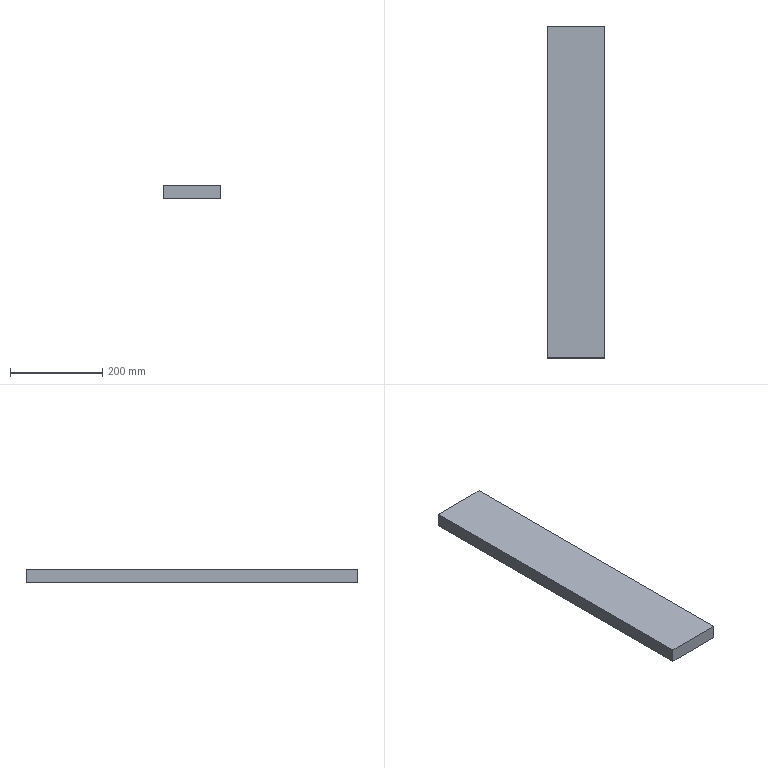Part | SolidWorks | features Extrusion 1 | 1 solid | 6 faces | box 125 x 718 x 30 mm | volume 2692500 mm3 | plane 6
STEP:
#1=CARTESIAN_POINT('',(0.,718.,0.));
#2=VERTEX_POINT('',#1);
#3=CARTESIAN_POINT('',(0.,0.,0.));
#4=VERTEX_POINT('',#3);
#5=CARTESIAN_POINT('',(0.,0.,0.));
#6=DIRECTION('',(0.,-1.,0.));
#7=VECTOR('',#6,1000.);
#8=LINE('',#5,#7);
#9=EDGE_CURVE('',#2,#4,#8,.T.);
#10=ORIENTED_EDGE('',*,*,#9,.T.);
#11=CARTESIAN_POINT('',(0.,0.,30.));
#12=VERTEX_POINT('',#11);
#13=CARTESIAN_POINT('',(0.,0.,30.));
#14=DIRECTION('',(0.,0.,-1.));
#15=VECTOR('',#14,1000.);
#16=LINE('',#13,#15);
#17=EDGE_CURVE('',#12,#4,#16,.T.);
#18=ORIENTED_EDGE('',*,*,#17,.F.);
#19=CARTESIAN_POINT('',(0.,718.,30.));
#20=VERTEX_POINT('',#19);
#21=CARTESIAN_POINT('',(0.,0.,30.));
#22=DIRECTION('',(0.,-1.,0.));
#23=VECTOR('',#22,1000.);
#24=LINE('',#21,#23);
#25=EDGE_CURVE('',#20,#12,#24,.T.);
#26=ORIENTED_EDGE('',*,*,#25,.F.);
#27=CARTESIAN_POINT('',(0.,718.,30.));
#28=DIRECTION('',(0.,0.,-1.));
#29=VECTOR('',#28,1000.);
#30=LINE('',#27,#29);
#31=EDGE_CURVE('',#20,#2,#30,.T.);
#32=ORIENTED_EDGE('',*,*,#31,.T.);
#33=EDGE_LOOP('',(#10,#18,#26,#32));
#34=FACE_OUTER_BOUND('',#33,.T.);
#35=CARTESIAN_POINT('',(0.,0.,30.));
#36=DIRECTION('',(1.,0.,0.));
#37=DIRECTION('',(0.,0.,-1.));
#38=AXIS2_PLACEMENT_3D('',#35,#36,#37);
#39=PLANE('',#38);
#40=ADVANCED_FACE('',(#34),#39,.F.);
#41=CARTESIAN_POINT('',(125.,0.,0.));
#42=VERTEX_POINT('',#41);
#43=CARTESIAN_POINT('',(0.,0.,0.));
#44=DIRECTION('',(1.,0.,0.));
#45=VECTOR('',#44,1000.);
#46=LINE('',#43,#45);
#47=EDGE_CURVE('',#4,#42,#46,.T.);
#48=ORIENTED_EDGE('',*,*,#47,.T.);
#49=CARTESIAN_POINT('',(125.,0.,30.));
#50=VERTEX_POINT('',#49);
#51=CARTESIAN_POINT('',(125.,0.,30.));
#52=DIRECTION('',(0.,0.,-1.));
#53=VECTOR('',#52,1000.);
#54=LINE('',#51,#53);
#55=EDGE_CURVE('',#50,#42,#54,.T.);
#56=ORIENTED_EDGE('',*,*,#55,.F.);
#57=CARTESIAN_POINT('',(0.,0.,30.));
#58=DIRECTION('',(1.,0.,0.));
#59=VECTOR('',#58,1000.);
#60=LINE('',#57,#59);
#61=EDGE_CURVE('',#12,#50,#60,.T.);
#62=ORIENTED_EDGE('',*,*,#61,.F.);
#63=ORIENTED_EDGE('',*,*,#17,.T.);
#64=EDGE_LOOP('',(#48,#56,#62,#63));
#65=FACE_OUTER_BOUND('',#64,.T.);
#66=CARTESIAN_POINT('',(0.,0.,30.));
#67=DIRECTION('',(0.,1.,0.));
#68=DIRECTION('',(0.,0.,1.));
#69=AXIS2_PLACEMENT_3D('',#66,#67,#68);
#70=PLANE('',#69);
#71=ADVANCED_FACE('',(#65),#70,.F.);
#72=CARTESIAN_POINT('',(125.,718.,0.));
#73=VERTEX_POINT('',#72);
#74=CARTESIAN_POINT('',(125.,0.,0.));
#75=DIRECTION('',(0.,1.,0.));
#76=VECTOR('',#75,1000.);
#77=LINE('',#74,#76);
#78=EDGE_CURVE('',#42,#73,#77,.T.);
#79=ORIENTED_EDGE('',*,*,#78,.T.);
#80=CARTESIAN_POINT('',(125.,718.,30.));
#81=VERTEX_POINT('',#80);
#82=CARTESIAN_POINT('',(125.,718.,30.));
#83=DIRECTION('',(0.,0.,-1.));
#84=VECTOR('',#83,1000.);
#85=LINE('',#82,#84);
#86=EDGE_CURVE('',#81,#73,#85,.T.);
#87=ORIENTED_EDGE('',*,*,#86,.F.);
#88=CARTESIAN_POINT('',(125.,0.,30.));
#89=DIRECTION('',(0.,1.,0.));
#90=VECTOR('',#89,1000.);
#91=LINE('',#88,#90);
#92=EDGE_CURVE('',#50,#81,#91,.T.);
#93=ORIENTED_EDGE('',*,*,#92,.F.);
#94=ORIENTED_EDGE('',*,*,#55,.T.);
#95=EDGE_LOOP('',(#79,#87,#93,#94));
#96=FACE_OUTER_BOUND('',#95,.T.);
#97=CARTESIAN_POINT('',(125.,0.,30.));
#98=DIRECTION('',(-1.,0.,0.));
#99=DIRECTION('',(0.,0.,1.));
#100=AXIS2_PLACEMENT_3D('',#97,#98,#99);
#101=PLANE('',#100);
#102=ADVANCED_FACE('',(#96),#101,.F.);
#103=CARTESIAN_POINT('',(0.,718.,0.));
#104=DIRECTION('',(-1.,0.,0.));
#105=VECTOR('',#104,1000.);
#106=LINE('',#103,#105);
#107=EDGE_CURVE('',#73,#2,#106,.T.);
#108=ORIENTED_EDGE('',*,*,#107,.T.);
#109=ORIENTED_EDGE('',*,*,#31,.F.);
#110=CARTESIAN_POINT('',(0.,718.,30.));
#111=DIRECTION('',(-1.,0.,0.));
#112=VECTOR('',#111,1000.);
#113=LINE('',#110,#112);
#114=EDGE_CURVE('',#81,#20,#113,.T.);
#115=ORIENTED_EDGE('',*,*,#114,.F.);
#116=ORIENTED_EDGE('',*,*,#86,.T.);
#117=EDGE_LOOP('',(#108,#109,#115,#116));
#118=FACE_OUTER_BOUND('',#117,.T.);
#119=CARTESIAN_POINT('',(0.,718.,30.));
#120=DIRECTION('',(0.,-1.,0.));
#121=DIRECTION('',(0.,0.,-1.));
#122=AXIS2_PLACEMENT_3D('',#119,#120,#121);
#123=PLANE('',#122);
#124=ADVANCED_FACE('',(#118),#123,.F.);
#125=ORIENTED_EDGE('',*,*,#25,.T.);
#126=ORIENTED_EDGE('',*,*,#61,.T.);
#127=ORIENTED_EDGE('',*,*,#92,.T.);
#128=ORIENTED_EDGE('',*,*,#114,.T.);
#129=EDGE_LOOP('',(#125,#126,#127,#128));
#130=FACE_OUTER_BOUND('',#129,.T.);
#131=CARTESIAN_POINT('',(0.,0.,30.));
#132=DIRECTION('',(0.,0.,-1.));
#133=DIRECTION('',(-1.,0.,0.));
#134=AXIS2_PLACEMENT_3D('',#131,#132,#133);
#135=PLANE('',#134);
#136=ADVANCED_FACE('',(#130),#135,.F.);
#137=ORIENTED_EDGE('',*,*,#9,.F.);
#138=ORIENTED_EDGE('',*,*,#107,.F.);
#139=ORIENTED_EDGE('',*,*,#78,.F.);
#140=ORIENTED_EDGE('',*,*,#47,.F.);
#141=EDGE_LOOP('',(#137,#138,#139,#140));
#142=FACE_OUTER_BOUND('',#141,.T.);
#143=CARTESIAN_POINT('',(0.,0.,0.));
#144=DIRECTION('',(0.,0.,-1.));
#145=DIRECTION('',(-1.,0.,0.));
#146=AXIS2_PLACEMENT_3D('',#143,#144,#145);
#147=PLANE('',#146);
#148=ADVANCED_FACE('',(#142),#147,.T.);
#149=CLOSED_SHELL('',(#40,#71,#102,#124,#136,#148));
#150=MANIFOLD_SOLID_BREP('',#149);
#151=CARTESIAN_POINT('',(0.,0.,0.));
#152=DIRECTION('',(0.,0.,1.));
#153=DIRECTION('',(1.,0.,0.));
#154=AXIS2_PLACEMENT_3D('',#151,#152,#153);
#155=(LENGTH_UNIT()NAMED_UNIT(*)SI_UNIT(.MILLI.,.METRE.));
#156=UNCERTAINTY_MEASURE_WITH_UNIT(LENGTH_MEASURE(0.00001),#155,'','');
#157=(NAMED_UNIT(*)PLANE_ANGLE_UNIT()SI_UNIT($,.RADIAN.));
#158=(NAMED_UNIT(*)SI_UNIT($,.STERADIAN.)SOLID_ANGLE_UNIT());
#159=(GEOMETRIC_REPRESENTATION_CONTEXT(3)GLOBAL_UNCERTAINTY_ASSIGNED_CONTEXT((#156))GLOBAL_UNIT_ASSIGNED_CONTEXT((#155,#157,#158))REPRESENTATION_CONTEXT('',''));
#160=ADVANCED_BREP_SHAPE_REPRESENTATION('',(#150,#154),#159);